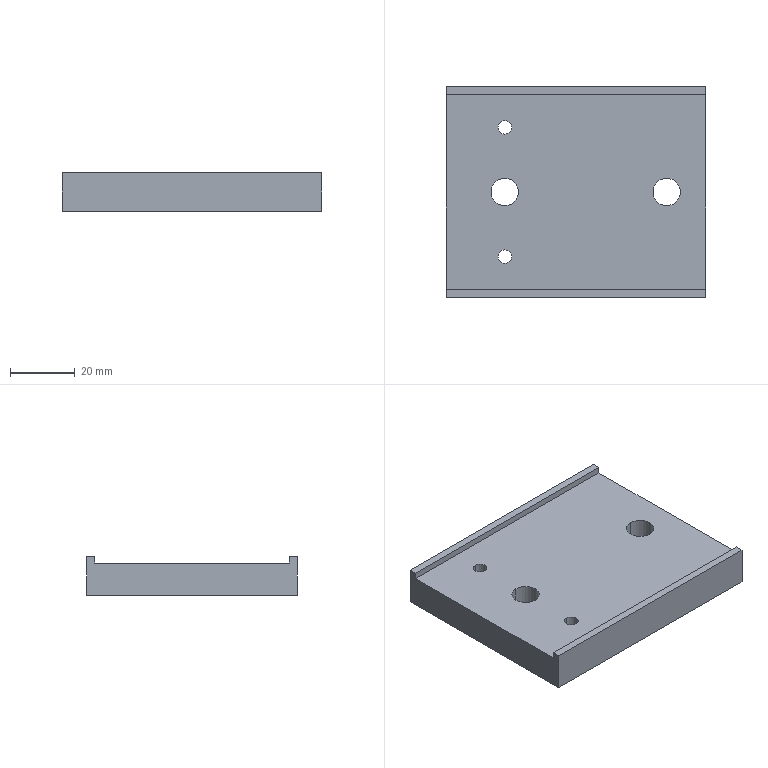NC program | NX | posted with a generic post | part box 80 x 65 x 12 mm
Whole program:
N10 G17 G21 G94 G90
(DRILLING_COPY_1 , TOOL : D6A45)
N12 T07 M6
N14 G54
N16 G17 G0 G90 X-22. Y-20. S3000 M3
N18 G43 Z30. H7
N20 G94 G81 G98 Z-3. F200. R1.
N22 Y0.
N24 Y20.
N26 X28. Y0.
N28 G80
N30 G0 X28. Y0. Z30.
N32 M5
(DRILLING_COPY_1_COPY , TOOL : 4.2ZT)
N34 T14 M6
N36 G54
N38 G17 G0 G90 X-22. Y-20. S2000 M3
N40 G43 Z30. H14
N42 G94 G83 G98 Z-14.762 F200. Q2. R1.
N44 Y20.
N46 G80
N48 G0 X-22. Y20. Z30.
N50 M5
(DRILLING_COPY_1_COPY_COPY , TOOL : 8.5ZT)
N52 T08 M6
N54 G54
N56 G17 G0 G90 X28. Y0. S2000 M3
N58 G43 Z30. H8
N60 G94 G83 G98 Z-16.054 F200. Q2. R1.
N62 X-22.
N64 G80
N66 G0 X-22. Y0. Z30.
N68 M5
(ZLEVEL_PROFILE_1_COPY_1_COPY_COPY_1_COPY , TOOL : D6A45)
N70 T07 M6
N72 G54
N74 G17 G0 G90 X-40.923 Y34.497 S7500 M3
N76 G43 Z30. H7
N78 Z0.
N80 G94 G1 Z-1. F1000.
N82 X-40.521 Y33.8
N84 G3 X-40.001 Y33.5 R0.6
N86 G1 X40.001
N88 G2 X41. Y32.501 R0.999
N90 G1 Y29.999
N92 G2 X40.001 Y29. R0.999
N94 G1 X-40.001
N96 G2 X-41. Y29.999 R0.999
N98 G1 Y32.501
N100 G2 X-40.001 Y33.5 R0.999
N102 G3 X-39.481 Y33.8 R0.6
N104 G1 X-38.962 Y34.7
N106 Z0.
N108 G0 Z30.
N110 X40.923 Y-34.497
N112 Z0.
N114 G1 Z-1.
N116 X40.521 Y-33.8
N118 G3 X40.001 Y-33.5 R0.6
N120 G1 X-40.001
N122 G2 X-41. Y-32.501 R0.999
N124 G1 Y-29.999
N126 G2 X-40.001 Y-29. R0.999
N128 G1 X40.001
N130 G2 X41. Y-29.999 R0.999
N132 G1 Y-32.501
N134 G2 X40.001 Y-33.5 R0.999
N136 G3 X39.481 Y-33.8 R0.6
N138 G1 X38.962 Y-34.7
N140 Z0.
N142 G0 Z30.
(刀补11 , TOOL : D10JING)
N144 T11 M6
N146 G17 G43 G0 G90 X46.478 Y23.356 Z30. S7500 H11 M3
N148 Z-0.5
N150 G94 G1 Z-2. F1100.
N152 G41 X46.443 Y23.45 D11
N154 X45.866 Y24.45
N156 G3 X45. Y24.95 R1.
N158 G1 X-45.
N160 G3 X-45.866 Y24.45 R1.
N162 G1 X-46.443 Y23.45
N164 G40
N166 X-46.478 Y23.356
N168 Z-0.5
N170 G0 Z1.1
N172 G1 Y-23.356 F6000.
N174 G0 Z-0.5
N176 G1 Z-2. F1100.
N178 G41 X-46.443 Y-23.45
N180 X-45.866 Y-24.45
N182 G3 X-45. Y-24.95 R1.
N184 G1 X45.
N186 G3 X45.866 Y-24.45 R1.
N188 G1 X46.443 Y-23.45
N190 G40
N192 X46.478 Y-23.356
N194 Z-0.5
N196 G0 Z30.
N198 M5
N200 M2